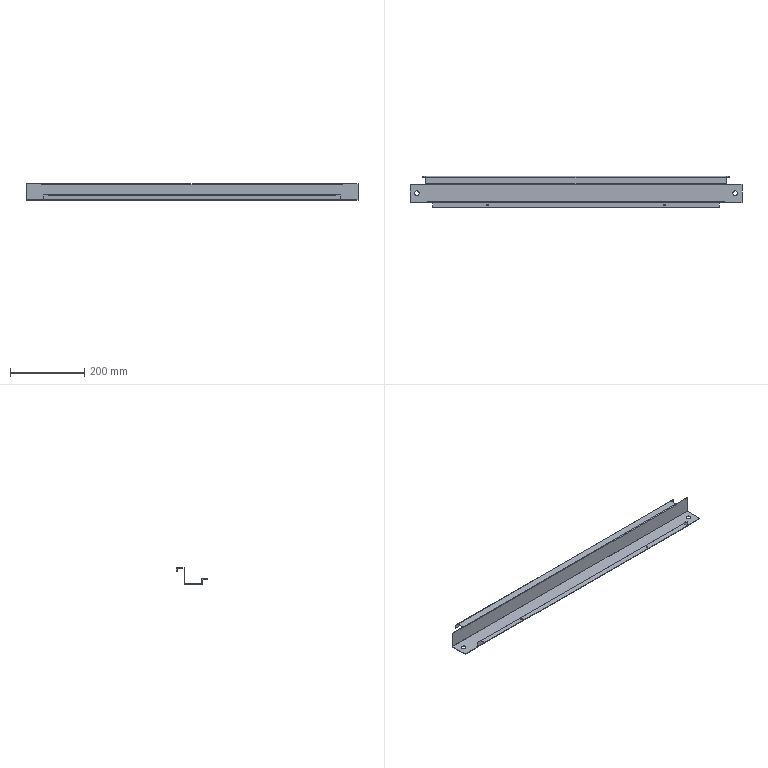Part | SolidWorks | features EdgeFlange 5, ICE 2, SMBaseFlange 2, FlatPattern 1, SheetMetal 1 | 1 solid | 86 faces | box 897 x 84 x 45 mm | volume 190615 mm3 | plane 68 | cylinder 18 | commonest cylinder face diameters 0.2 x5 3.2 x5 5.1 x4 13 x4